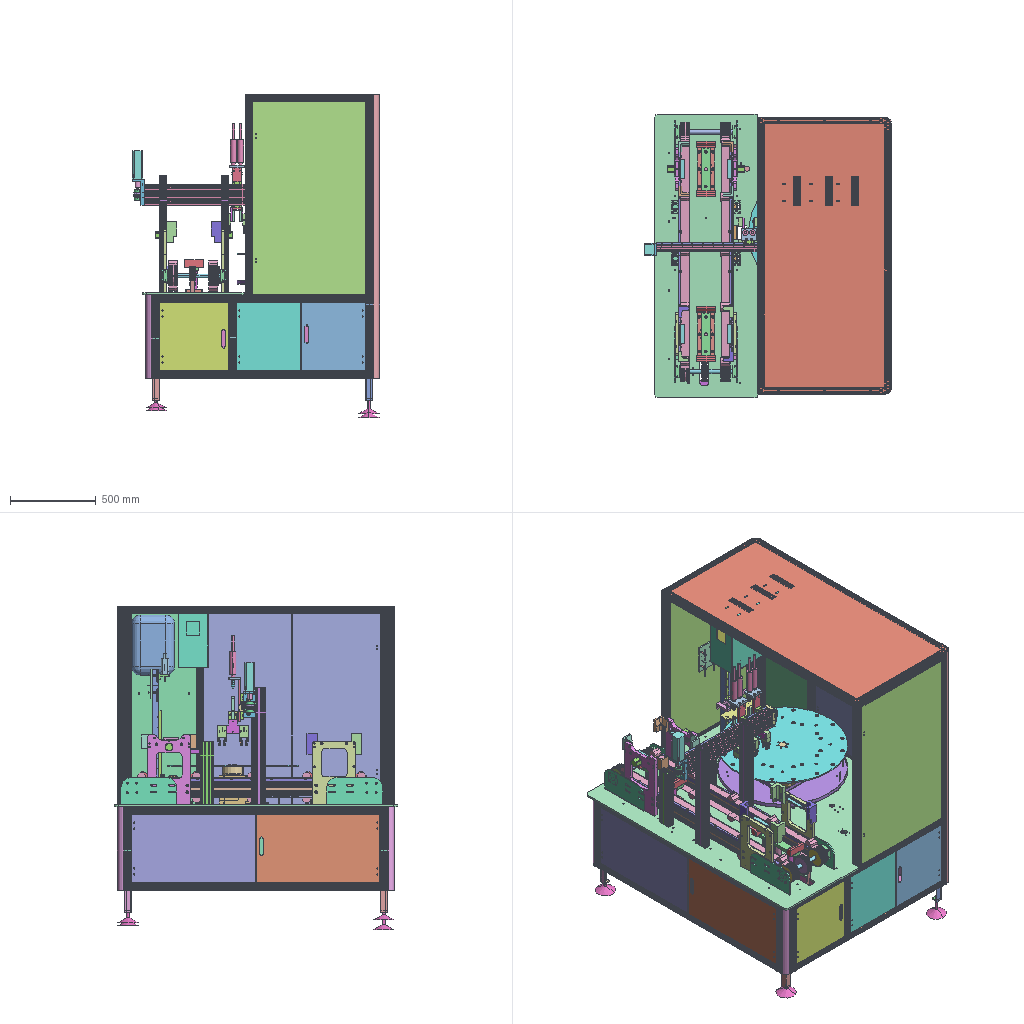Assembly | SolidWorks | 147 different items | 355 placed | box 1437 x 1650 x 1881 mm
Parts list (item | name | quantity | parent item):
1 | 1121x512x10 | x2 | in 72
2 | 1121x654x10 | x2 | in 72
3 | 12X20带轮外购加工件 | x2 | in 145, 146
4 | 12X65轴HL-TSJKD-03.3-2.1-2 | x1 | in 146
5 | 12X80轴HL-TSJKD-03.3-2.1-1 | x1 | in 145
6 | 6205轴承-外购件 | x8 | in 18, 20
7 | 6205轴承座-外购件 | x4 | in 18, 20
8 | 80DF+0.55KW普通电机+050减速机(2018-5-28)  (subassembly) | x1 | in 72
9 | 80DF+0.55KW普通电机+050减速机(2018-5-28) .stp (subassembly) | x1 | -
10 | 80针HL-TSJKD-04.4-5 | x8 | in 86
11 | CDM2B20-100Z-XC8B双杆双作用气缸-外购件 | x4 | in 79
12 | DNCJ 32X35-20-PPV-A气缸-外购件 | x1 | in 86
13 | DNCJ 32X60-20-PPV-A气缸外购件 | x1 | in 86
14 | HL-TSJKD-02.1工作台框架 (subassembly) | x1 | in 72
15 | MHZ2-20D-M9BW气缸 -外购件 | x8 | in 80, 81
16 | 三针绝缘板HL-TSJKD-04.4-1 | x1 | in 86
17 | 上料系统HL-TSJKD-03 (subassembly) | x1 | -
18 | 主动部件装配HL-TSJKD-03.1-2 (subassembly) | x1 | in 17
19 | 从动轴-353HL-TSJKD-03.1-3.1 | x1 | in 20
20 | 从动部件HL-TSJKD-03.1-3 (subassembly) | x1 | in 17
21 | 传动组件装配HL-TSJKD-03.3-2.2 (subassembly) | x2 | in 81
22 | 伺服电机-外购件ECMA-C20604RS带刹车带油封 | x1 | in 145
23 | 伺服电机联轴器-外购件 | x1 | in 145
24 | 储物柜侧门HL-TSJKD-02.5-4 | x1 | in 72
25 | 储物柜右柜门HL-TSJKD-02.5-3 | x1 | in 72
26 | 储物柜左柜门HL-TSJKD-02.5-2 | x1 | in 72
27 | 储物柜柜体HL-TSJKD-02.5-1 | x1 | in 72
28 | 光圆HL-TSJKD-03.2-2.2-3 | x4 | in 52
29 | 光敏柜柜体HL-TSJKD-02.4-1 | x1 | in 72
30 | 光敏柜盖板HL-TSJKD-02.4-2 | x1 | in 72
31 | 包电柜右门HL-TSJKD-02.8-3 | x1 | in 147
32 | 包电柜左门HL-TSJKD-02.8-2 | x1 | in 147
33 | 包电柜柜体HL-TSJKD-02.8-1 | x1 | in 147
34 | 半圆弧铝型材-1650HL-TSJKD-02.1-2.11 | x2 | in 128
35 | 半圆弧铝型材-485HL-TSJKD-02.1-2.12 | x2 | in 128
36 | 压力表盖板HL-TSJKD-02.9-2 | x1 | in 72
37 | 压皮带块1HL-TSJKD-03.3-5.1 | x2 | in 81
38 | 压皮带块2-1HL-TSJKD-03.3-5.2-1(2) | x2 | in 40
39 | 压皮带块2-2HL-TSJKD-03.3-5.2-2 | x2 | in 40
40 | 压皮带块2装配HL-TSJKD-03.3-5.2 (subassembly) | x2 | in 81
41 | 去油毛刷支架HL-TSJKD-06.2 | x10 | in 88
42 | 同步带HTD5M-3200-48-外购加工件  | x2 | in 17
43 | 同步带（HTD 750-5m）-外购件 | x1 | in 17
44 | 同步轮5m-af-30齿-27 | x1 | in 107
45 | 同步轮5m-af-70齿-27-外购加工件 | x1 | in 18
46 | 同步轮5m-af-70齿-50-外购加工件 | x2 | in 18
47 | 同步轮5m-af-70齿-50无键槽-外购加工件 | x2 | in 20
48 | 喇叭脚 | x4 | in 72
49 | 圆盘HL-TSJKD-05.1 | x1 | in 51
50 | 圆盘支撑HL-TSJKD-05.2 | x1 | in 51
51 | 圆盘机构HL-TSJKD-05 (subassembly) | x1 | -
52 | 塑料盆导向托架装配HL-TSJKD-03.2-2.2 (subassembly) | x2 | in 17
53 | 塑料盆搭扣HL-TSJKD-03.2-2.1 (subassembly) | x4 | in 17
54 | 塑料盆搭扣体HL-TSJKD-03.2-2.1-1 | x4 | in 53
55 | 塑料盆搭扣座HL-TSJKD-03.2-2.1-3 | x8 | in 53
56 | 塑料盆搭扣轴HL-TSJKD-03.2-2.1-2 | x4 | in 53
57 | 夹爪HL-TSJKD-03.3-4.1 | x14 | in 80
58 | 夹爪橡胶套-外购件 | x14 | in 80
59 | 实体1.stp | x1 | -
60 | 实体2.stp | x1 | -
61 | 实体3.stp | x1 | -
62 | 实体4.stp | x1 | -
63 | 导轨216.5HL-TSJKD-03.3-3.5 | x4 | in 85
64 | 导轨720HL-TSJKD-03.3-2.2-1 | x2 | in 21
65 | 导轨固定架HL-TSJKD-03.3-3.3 | x2 | in 85
66 | 尼龙导向角HL-TSJKD-03.2-3.1-1 | x2 | in 17
67 | 尼龙导向角切口HL-TSJKD-03.2-3.1-3 | x2 | in 17
68 | 尼龙导向角切口镜像HL-TSJKD-03.2-3.1-4 | x2 | in 17
69 | 尼龙导向角镜像HL-TSJKD-03.2-3.1-2 | x2 | in 17
70 | 尼龙托板HL-TSJKD-03.1-1.5 | x4 | in 17
71 | 工作台气缸固定板HL-TSJKD-02.3 | x2 | in 72
72 | 工作台装配体HL-TSJKD-02 (subassembly) | x1 | in 17
73 | 工作台铝板（底板）HL-TSJKD-02.2 | x1 | in 72
74 | 带轮固定板1HL-TSJKD-03.3-1.4 | x1 | in 120
75 | 带轮固定板2HL-TSJKD-03.3-1.5 | x1 | in 120
76 | 悬挂油箱盖板HL-TSJKD-02.9-1 | x1 | in 72
77 | 托架导向HL-TSJKD-03.2-2.2-2 | x4 | in 52
78 | 托架导向座HL-TSJKD-03.2-2.2-1 | x2 | in 52
79 | 执行件 (subassembly) | x4 | in 81
80 | 执行末端HL-TSJKD-03.3-4 (subassembly) | x7 | in 81
81 | 抓取机构HL-TSJKD-03.3 (subassembly) | x1 | in 17
82 | 抓取立柱铝型材80X40-680HL-TSJKD-03.3-1.1 | x2 | in 120
83 | 抓取部件1HL-TSJKD-03.3-3.2 | x2 | in 85
84 | 抓取部件HL-TSJKD-03.3-3.1 | x2 | in 85
85 | 抓取部分HL-TSJKD-03.3-3 (subassembly) | x2 | in 81
86 | 检测跳火工装HL-TSJKD-04 (subassembly) | x1 | -
87 | 毛刷托盘HL-TSJKD-06.1 | x1 | in 88
88 | 毛刷机构HL-TSJKD-06 (subassembly) | x1 | -
89 | 气缸-SDA 25X20-B-外购件 | x2 | in 17
90 | 气缸DNC50x230 PPV A-外购件 | x2 | in 17
91 | 气缸固定架HL-TSJKD-03.3-3.4 | x4 | in 85
92 | 气缸垫块HL-TSJKD-04.3-2 | x2 | in 86
93 | 油杯HL-TSJKD-04.5-2 | x4 | in 86
94 | 油杯托槽HL-TSJKD-04.5-1 | x1 | in 86
95 | 油槽托架HL-TSJKD-04.2-1 | x2 | in 86
96 | 油箱-304加厚方型10L0.8厚-外购件 | x1 | -
97 | 油箱-304加厚方型20L0.8厚-外购件 | x1 | -
98 | 油箱右柜门HL-TSJKD-02.7-1 | x1 | in 72
99 | 油箱左柜门HL-TSJKD-02.7-2 | x1 | in 72
100 | 浮动接头-外购件 FJ1008 M8x1.25 | x4 | in 79
101 | 滑块-外购件（TRH15A直线导轨块） | x12 | in 21, 85, 86
102 | 滑块支座HL-TSJKD-04.3-1 | x2 | in 86
103 | 电机ECM-B3M-C20604RS1-外购件 | x1 | in 107
104 | 电机支架1HL-TSJKD-03.1-4.1-1 | x2 | in 106
105 | 电机支架2HL-TSJKD-03.1-4.1-2 | x1 | in 106
106 | 电机支架HL-TSJKD-03.1-4.1 (subassembly) | x1 | in 107
107 | 电机组件HL-TSJKD-03.1-4 (subassembly) | x1 | in 17
108 | 电极头HL-TSJKD-04.4-6 | x4 | in 86
109 | 电极头触点导电块HL-TSJKD-04.4-7 | x4 | in 86
110 | 电极座HL-TSJKD-04.4-4 | x8 | in 86
111 | 电气柜右柜体HL-TSJKD-02.6-1.2 | x1 | in 72
112 | 电气柜右柜门HL-TSJKD-02.6-3.DWG | x2 | in 72
113 | 电气柜左柜体HL-TSJKD-02.6-1.1 | x1 | in 72
114 | 电气柜左柜门HL-TSJKD-02.6-2 | x2 | in 72
115 | 直线轴承装配 (subassembly) | x4 | in 17
116 | 直线轴承轴 | x4 | in 115
117 | 直线轴承轴座-25&35x130有肩轴套（浙江茅）- | x4 | in 115
118 | 立式KP001轴承套-外购件 | x4 | in 120
119 | 立柱铝型材HL-TSJKD-04.1 | x1 | in 86
120 | 结构框架装配HL-TSJKD-03.3-1 (subassembly) | x1 | in 81
121 | 绝缘卡件HL-TSJKD-04.4-3.2 | x2 | in 123
122 | 绝缘板HL-TSJKD-04.4-3.1 | x1 | in 123
123 | 绝缘板部件HL-TSJKD-04.4-3 (subassembly) | x1 | in 86
124 | 角铁框架HL-TSJKD-02.1-1 | x1 | in 14
125 | 跳火导轨495-外购加工件（配合TRH15A） | x2 | in 86
126 | 轴-353HL-TSJKD-03.1-2.1 | x1 | in 18
127 | 轴承安装板HL-TSJKD-03.1-1.6 | x4 | in 17
128 | 铝合金框架装配HL-TSJKD-02.1-2 (subassembly) | x1 | in 14
129 | 铝型材40X40-1125HL-TSJKD-02.1-2.1 | x1 | in 128
130 | 铝型材40X40-1164HL-TSJKD-02.1-2.2 | x2 | in 128
131 | 铝型材40X40-1200HL-TSJKD-02.1-2.3 | x4 | in 128
132 | 铝型材40X40-1450HL-TSJKD-02.1-2.4 | x5 | in 128
133 | 铝型材40X40-1530HL-TSJKD-02.1-2.5 | x1 | in 128
134 | 铝型材40X40-1650HL-TSJKD-02.1-2.6 | x4 | in 128
135 | 铝型材40X40-170HL-TSJKD-02.1-2.7 | x3 | in 128
136 | 铝型材40X40-405HL-TSJKD-02.1-2.8 | x2 | in 128
137 | 铝型材40X40-485HL-TSJKD-02.1-2.9 | x4 | in 128
138 | 铝型材40X40-658HL-TSJKD-02.1-2.10 | x2 | in 128
139 | 铝型材40x120-720HL-TSJKD-03.3-1.2 | x1 | in 120
140 | 铝型材80X40-1260HL-TSJKD-03.1-1.4 | x2 | in 17
141 | 铝型材80X40-366HL-TSJKD-03.1-1.3 | x2 | in 17
142 | 铝板366x250x20HL-TSJKD-03.1-1.2 | x2 | in 17
143 | 铝板406X250X20HL-TSJKD-03.1-1.1 | x2 | in 17
144 | 顶部盖板HL-TSJKD-02.9-3 | x1 | in 72
145 | 驱动源主动部件装配HL-TSJKD-03.3-2.1 (subassembly) | x1 | in 81
146 | 驱动源从动部件装配HL-TSJKD-03.3-2.1 (subassembly) | x1 | in 81
147 | 高压包电柜装配HL-TSJKD-02.8 (subassembly) | x1 | in 72
Mates (type | each side: item.copy, entity, surface, feature), first 515 of 572 lines:
In the top assembly
Coincident | 73.1 face plane 凸台-拉伸1 | 119.1 face plane 凸台-拉伸1 | 2 times
DistanceDim | 119.1 face plane 凸台-拉伸2 | 73.1 face plane 凸台-拉伸1
DistanceDim | 73.1 face plane 凸台-拉伸1 | 87.1 face plane 凸台-拉伸1
Concentric | 49.1 face cylinder 凸台-拉伸1 | 87.1 face cylinder 边线-法兰1
Coincident | 124.1 edge | 97.1 face plane 凸台-拉伸1
Coincident | 124.1 face plane 等边角钢gb／t 9787-1988 40X40X5 型号：4#(1) | 97.1 face plane 凸台-拉伸1 | 2 times
Coincident | 76.1 face plane 基体-法兰1 | 96.1 face plane 凸台-拉伸1
Coincident | 76.1 face plane 边线-法兰1 | 96.1 face plane 凸台-拉伸1
In subassembly 88
Coincident | 87.2 face plane 切除-拉伸1 | 41.1 face plane 凸台-拉伸1 | 3 times
Coincident | 87.2 face plane 切除-拉伸1 | 41.2 face plane 凸台-拉伸1 | 3 times
In subassembly 17
Coincident | 73.2 face plane 凸台-拉伸1 | 142.1 face plane 凸台-拉伸1
Concentric | 73.2 face cylinder 凸台-拉伸1 | 142.1 face cylinder M8 螺纹孔2 | 2 times
Coincident | 73.2 face plane 凸台-拉伸1 | 142.2 face plane 凸台-拉伸1
Concentric | 73.2 face cylinder 凸台-拉伸1 | 142.2 face cylinder M8 螺纹孔2 | 2 times
Coincident | 73.2 face plane 凸台-拉伸1 | 143.1 face plane 切除-拉伸5
Coincident | 73.2 face plane 凸台-拉伸1 | 143.2 face plane 切除-拉伸5
Concentric | 73.2 face cylinder 凸台-拉伸1 | 143.2 face cylinder M8 螺纹孔4 | 2 times
Concentric | 73.2 face cylinder 凸台-拉伸1 | 143.1 face cylinder M8 螺纹孔4 | 2 times
Coincident | 73.2 face plane 凸台-拉伸1 | 127.1 face plane 凸台-拉伸2
Coincident | 142.1 face plane 凸台-拉伸1 | 127.1 face plane 凸台-拉伸1
Slot | 127.1 face plane 切除-拉伸1 | 142.1 face cylinder M8 螺纹孔1
Coincident | 73.2 face plane 凸台-拉伸1 | 127.2 face plane 凸台-拉伸2
Coincident | 142.2 face plane 凸台-拉伸1 | 127.2 face plane 凸台-拉伸1
Slot | 142.2 face cylinder M8 螺纹孔1 | 127.2 face plane 切除-拉伸1
Coincident | 127.1 face plane 凸台-拉伸2 | 127.2 face plane 凸台-拉伸2
Coincident | 73.2 face plane 凸台-拉伸1 | 127.3 face plane 凸台-拉伸2
Coincident | 73.2 face plane 凸台-拉伸1 | 127.4 face plane 凸台-拉伸2
Coincident | 143.1 face plane 凸台-拉伸1 | 127.4 face plane 凸台-拉伸1
Coincident | 143.2 face plane 凸台-拉伸1 | 127.3 face plane 凸台-拉伸1
Slot | 127.3 face plane 切除-拉伸1 | 143.2 face cylinder M8 螺纹孔3
Coincident | 127.4 face plane 凸台-拉伸2 | 127.3 face plane 凸台-拉伸2
Slot | 127.4 face plane 切除-拉伸1 | 143.1 face cylinder M8 螺纹孔3
Coincident | 142.2 face plane 凸台-拉伸1 | 140.1 face plane 凸台-拉伸1
Coincident | 143.1 face plane 凸台-拉伸1 | 140.2 face plane 凸台-拉伸1
Coincident | 143.2 face plane 凸台-拉伸1 | 140.1 face plane 凸台-拉伸1
DistanceDim | 140.1 face plane 凸台-拉伸1 | 143.2 face plane 凸台-拉伸1
Coincident | 140.2 face plane 凸台-拉伸1 | 140.1 face plane 凸台-拉伸1 | 2 times
Tangent | 143.2 face cylinder 打孔尺寸(%根据)内六角圆柱头螺钉的类型1 | 140.1 face plane 凸台-拉伸1
Coincident | 140.2 face plane 凸台-拉伸1 | 70.1 face plane 凸台-拉伸1
Coincident | 140.1 edge | 70.1 edge
Tangent | 140.1 face plane 凸台-拉伸1 | 70.1 face cylinder 打孔尺寸(%根据)内六角圆柱头螺钉的类型1
Coincident | 70.2 edge | 70.1 edge
Coincident | 70.2 face plane 凸台-拉伸1 | 70.1 face plane 凸台-拉伸1
Parallel | 140.2 face plane 凸台-拉伸1 | 70.3 face plane 凸台-拉伸1
Coincident | 140.2 face plane 凸台-拉伸1 | 70.3 face plane 凸台-拉伸1
Tangent | 140.2 face plane 凸台-拉伸1 | 70.3 face cylinder 打孔尺寸(%根据)内六角圆柱头螺钉的类型1
Coincident | 140.2 edge | 70.3 edge
Coincident | 70.4 edge | 70.3 edge
Coincident | 70.3 face plane 凸台-拉伸1 | 70.4 face plane 凸台-拉伸1
Coincident | 141.1 face plane 凸台-拉伸1 | 141.2 face plane 凸台-拉伸1 | 2 times
Coincident | 140.1 face plane 凸台-拉伸1 | 141.2 face plane 凸台-拉伸1
Coincident | 140.2 face plane 凸台-拉伸1 | 141.1 face plane 凸台-拉伸1
Coincident | 73.2 face plane 凸台-拉伸1 | 141.1 face plane 凸台-拉伸1
DistanceDim | 141.1 face plane 凸台-拉伸1 | 143.1 face plane 凸台-拉伸1
Coincident | 70.4 face plane 凸台-拉伸1 | 42.1 face plane 凸台-拉伸1
Coincident | 127.1 face plane 凸台-拉伸1 | 7.1 face plane 凸台-拉伸1
Concentric | 127.1 face cylinder 切除-拉伸1 | 7.1 face cylinder M8 六角头螺栓的柱形沉头孔1 | 2 times
Concentric | 127.2 face cylinder 切除-拉伸1 | 7.2 face cylinder M8 六角头螺栓的柱形沉头孔1 | 2 times
Concentric | 42.2 face cylinder 凸台-拉伸1 | 46.1 face cylinder 凸台-拉伸2
Coincident | 127.3 face plane 凸台-拉伸1 | 7.3 face plane 凸台-拉伸1
Concentric | 127.3 face cylinder 切除-拉伸1 | 7.3 face cylinder M8 六角头螺栓的柱形沉头孔1 | 3 times
Concentric | 127.4 face cylinder 切除-拉伸1 | 7.4 face cylinder M8 六角头螺栓的柱形沉头孔1 | 2 times
Concentric | 42.1 face cylinder 凸台-拉伸1 | 47.1 face cylinder 凸台-拉伸3
DistanceDim | 42.1 face plane 凸台-拉伸1 | 46.2 face plane 凸台-拉伸3
Coincident | 73.2 face plane 凸台-拉伸1 | 105.1 face plane 基体-法兰1
Slot | 105.1 face plane 切除-拉伸1 | 73.2 face cylinder M8 螺纹孔1
Slot | 73.2 face cylinder M8 螺纹孔1 | 105.1 face plane 切除-拉伸1
Coincident | 45.1 face plane 凸台-拉伸3 | 44.1 face plane 凸台-拉伸2
Concentric | 143.2 face cylinder 切除-拉伸4 | 89.1 face cylinder 凸台-拉伸3
Coincident | 143.2 face plane 凸台-拉伸1 | 89.1 face plane 凸台-拉伸2
Concentric | 143.1 face cylinder 切除-拉伸4 | 89.2 face cylinder 凸台-拉伸3
Coincident | 143.1 face plane 凸台-拉伸1 | 89.2 face plane 凸台-拉伸2
Concentric | 71.1 face cylinder 凸台-拉伸1 | 90.1 face cylinder 凸台-拉伸4
Coincident | 71.1 face plane 凸台-拉伸1 | 90.1 face plane 凸台-拉伸1
Concentric | 71.2 face cylinder 凸台-拉伸1 | 90.2 face cylinder 凸台-拉伸4
Coincident | 71.2 face plane 凸台-拉伸1 | 90.2 face plane 凸台-拉伸1
Coincident | 142.2 face plane 凸台-拉伸1 | 55.1 face plane 凸台-拉伸1
Coincident | 142.1 face plane 凸台-拉伸1 | 55.2 face plane 凸台-拉伸1
Concentric | 142.2 face cylinder 切除-拉伸5 | 55.1 face cylinder M8 螺纹孔1
Concentric | 142.2 face cylinder 切除-拉伸5 | 55.3 face cylinder M8 螺纹孔1
Concentric | 142.1 face cylinder 切除-拉伸5 | 55.2 face cylinder M8 螺纹孔1
Concentric | 142.1 face cylinder 切除-拉伸5 | 55.4 face cylinder M8 螺纹孔1
Coincident | 143.1 face plane 凸台-拉伸1 | 54.1 face plane 切除-拉伸1
Concentric | 143.1 face cylinder 打孔尺寸(%根据)内六角圆柱头螺钉的类型3 | 55.5 face cylinder M8 螺纹孔1
Concentric | 143.1 face cylinder 打孔尺寸(%根据)内六角圆柱头螺钉的类型3 | 55.6 face cylinder M8 螺纹孔1
Coincident | 143.2 face plane 凸台-拉伸1 | 55.7 face plane 凸台-拉伸1
Concentric | 143.2 face cylinder 打孔尺寸(%根据)内六角圆柱头螺钉的类型3 | 55.7 face cylinder M8 螺纹孔1
Concentric | 143.2 face cylinder 打孔尺寸(%根据)内六角圆柱头螺钉的类型3 | 55.8 face cylinder M8 螺纹孔1
Concentric | 71.2 face cylinder 凸台-拉伸1 | 28.1 face cylinder 凸台-拉伸1
Concentric | 71.2 face cylinder 凸台-拉伸1 | 28.2 face cylinder 凸台-拉伸1
Coincident | 90.2 face plane 凸台-拉伸4 | 78.1 face plane 凸台-拉伸1
Concentric | 71.1 face cylinder 凸台-拉伸1 | 28.3 face cylinder 凸台-拉伸1
Concentric | 71.1 face cylinder 凸台-拉伸1 | 28.4 face cylinder 凸台-拉伸1
Coincident | 90.1 face plane 凸台-拉伸4 | 78.2 face plane 凸台-拉伸1
Coincident | 71.1 face plane 凸台-拉伸1 | 117.1 face plane 凸台-拉伸1
Concentric | 71.1 face cylinder M5 螺纹孔1 | 117.1 face cylinder M5 螺纹孔1 | 2 times
Coincident | 71.2 face plane 凸台-拉伸1 | 117.2 face plane 凸台-拉伸1
Coincident | 71.2 face plane 凸台-拉伸1 | 117.3 face plane 凸台-拉伸1
Coincident | 71.1 face plane 凸台-拉伸1 | 117.4 face plane 凸台-拉伸1
Concentric | 28.4 face cylinder 凸台-拉伸1 | 116.1 face cylinder 凸台-拉伸2
Concentric | 28.1 face cylinder 凸台-拉伸1 | 116.2 face cylinder 凸台-拉伸2
Concentric | 28.2 face cylinder 凸台-拉伸1 | 116.3 face cylinder 凸台-拉伸2
Concentric | 143.1 face cylinder M8 螺纹孔1 | 66.1 face cylinder 打孔尺寸(%根据)内六角圆柱头螺钉的类型2 | 2 times
Coincident | 143.1 face plane 凸台-拉伸1 | 66.1 face plane 切除-拉伸2
Concentric | 143.2 face cylinder M8 螺纹孔1 | 66.2 face cylinder 打孔尺寸(%根据)内六角圆柱头螺钉的类型2 | 2 times
Coincident | 143.2 face plane 凸台-拉伸1 | 66.2 face plane 切除-拉伸2
Concentric | 143.2 face cylinder M8 螺纹孔1 | 69.1 face cylinder 打孔尺寸(%根据)内六角圆柱头螺钉的类型2 | 2 times
Coincident | 143.2 face plane 凸台-拉伸1 | 69.1 face plane 切除-拉伸2
Concentric | 142.1 face cylinder M8 螺纹孔1 | 67.1 face cylinder 打孔尺寸(%根据)内六角圆柱头螺钉的类型3 | 2 times
Coincident | 142.1 face plane 凸台-拉伸1 | 67.1 face plane 切除-拉伸5
Concentric | 142.1 face cylinder M8 螺纹孔1 | 68.1 face cylinder 打孔尺寸(%根据)内六角圆柱头螺钉的类型3 | 2 times
Coincident | 142.1 face plane 凸台-拉伸1 | 68.1 face plane 切除-拉伸5
Concentric | 142.2 face cylinder M8 螺纹孔1 | 67.2 face cylinder 打孔尺寸(%根据)内六角圆柱头螺钉的类型3 | 2 times
Coincident | 142.2 face plane 凸台-拉伸1 | 67.2 face plane 切除-拉伸5
Concentric | 142.2 face cylinder M8 螺纹孔1 | 68.2 face cylinder 打孔尺寸(%根据)内六角圆柱头螺钉的类型3 | 2 times
Coincident | 142.2 face plane 凸台-拉伸1 | 68.2 face plane 切除-拉伸5
Coincident | 143.1 face plane 凸台-拉伸1 | 69.2 face plane 切除-拉伸2
Concentric | 143.1 face cylinder M8 螺纹孔1 | 69.2 face cylinder 打孔尺寸(%根据)内六角圆柱头螺钉的类型2 | 2 times
Coincident | 73.2 face plane 凸台-拉伸1 | 82.1 face plane 凸台-拉伸1
Coincident | 140.2 face plane 凸台-拉伸1 | 82.1 face plane 凸台-拉伸1
DistanceDim | 82.1 face plane 凸台-拉伸1 | 73.2 face plane 凸台-拉伸1
Concentric | 45.1 face cylinder 凸台-拉伸2 | 43.1 face cylinder 扫描1
DistanceDim | 43.1 face plane 扫描1 | 45.1 face plane 凸台-拉伸2
In subassembly 72
Coincident | 124.2 face plane 等边角钢gb／t 9787-1988 40X40X5 型号：4#(1) | 73.3 face plane 凸台-拉伸1 | 2 times
DistanceDim | 124.2 face plane 等边角钢gb／t 9787-1988 40X40X5 型号：4#(1) | 73.3 face plane 凸台-拉伸1
Coincident | 73.3 face plane 凸台-拉伸1 | 71.3 face plane 凸台-拉伸1
Coincident | 73.3 face plane 凸台-拉伸1 | 71.4 face plane 凸台-拉伸1
Concentric | 73.3 face cylinder M8 螺纹孔1 | 71.4 face cylinder 切除-拉伸1
Parallel | 73.3 face cylinder M8 螺纹孔1 | 71.4 face cylinder 凸台-拉伸1
Concentric | 73.3 face cylinder M8 螺纹孔1 | 71.3 face cylinder 凸台-拉伸1
Concentric | 73.3 face cylinder M8 螺纹孔1 | 71.3 face cylinder 切除-拉伸1
Coincident | 124.2 face plane 等边角钢gb／t 9787-1988 40X40X5 型号：4#(1) | 29.1 face plane 边线-法兰1
Coincident | 124.2 edge | 29.1 face plane 边线-法兰2
Coincident | 124.2 edge | 29.1 face plane 边线-法兰1
DistanceDim | 30.1 face plane 斜接法兰1 | 131.1 face plane 铝型材 40 X 40B X R4.5(1)
DistanceDim | 30.1 face plane 斜接法兰1 | 136.1 face plane 铝型材 40 X 40B X R4.5(1)
Coincident | 136.1 face plane 铝型材 40 X 40B X R4.5(1) | 30.1 face plane 基体-法兰1
Coincident | 124.2 face plane 等边角钢gb／t 9787-1988 40X40X5 型号：4#(1) | 27.1 face plane 基体-法兰1
Coincident | 124.2 edge | 27.1 face plane 边线-法兰1 | 2 times
Coincident | 26.1 face plane 基体-法兰1 | 25.1 face plane 基体-法兰1
Coincident | 26.1 face plane 斜接法兰1 | 25.1 face plane 斜接法兰1
DistanceDim | 26.1 face plane 斜接法兰1 | 131.2 face plane 铝型材 40 X 40B X R4.5(1)
DistanceDim | 26.1 face plane 斜接法兰1 | 136.2 face plane 铝型材 40 X 40B X R4.5(1)
DistanceDim | 25.1 face plane 斜接法兰1 | 134.1 face plane 铝型材 40 X 40B X R4.5(1)
Coincident | 26.1 face plane 基体-法兰1 | 24.1 face plane 基体-法兰1
Coincident | 26.1 face plane 斜接法兰1 | 24.1 face plane 斜接法兰1
DistanceDim | 24.1 face plane 斜接法兰1 | 137.1 face plane 铝型材 40 X 40B X R4.5(1)
Coincident | 124.2 face plane 等边角钢gb／t 9787-1988 40X40X5 型号：4#(1) | 113.1 face plane 基体-法兰1
Coincident | 124.2 edge | 113.1 face plane 边线-法兰1
Coincident | 124.2 edge | 113.1 face plane 基体-法兰1
Coincident | 124.2 edge | 111.1 face plane 基体-法兰1
Coincident | 124.2 face plane 等边角钢gb／t 9787-1988 40X40X5 型号：4#(1) | 111.1 face plane 基体-法兰1
DistanceDim | 29.1 face plane 基体-法兰1 | 111.1 face plane 基体-法兰1
DistanceDim | 112.1 face plane 斜接法兰1 | 137.2 face plane 铝型材 40 X 40B X R4.5(1)
DistanceDim | 112.1 face plane 斜接法兰1 | 132.1 face plane 铝型材 40 X 40B X R4.5(1)
Coincident | 137.2 face plane 铝型材 40 X 40B X R4.5(1) | 112.1 face plane 基体-法兰1
Coincident | 132.2 face plane 铝型材 40 X 40B X R4.5(1) | 112.2 face plane 基体-法兰1
DistanceDim | 112.2 face plane 斜接法兰1 | 134.2 face plane 铝型材 40 X 40B X R4.5(1)
DistanceDim | 112.2 face plane 斜接法兰1 | 132.3 face plane 铝型材 40 X 40B X R4.5(1)
Coincident | 137.3 face plane 铝型材 40 X 40B X R4.5(1) | 114.1 face plane 基体-法兰1
DistanceDim | 114.1 face plane 斜接法兰1 | 137.3 face plane 铝型材 40 X 40B X R4.5(1)
DistanceDim | 114.1 face plane 斜接法兰1 | 132.1 face plane 铝型材 40 X 40B X R4.5(1)
Coincident | 134.3 face plane 铝型材 40 X 40B X R4.5(1) | 114.2 face plane 基体-法兰1
DistanceDim | 114.2 face plane 斜接法兰1 | 134.3 face plane 铝型材 40 X 40B X R4.5(1)
DistanceDim | 114.2 face plane 斜接法兰1 | 132.3 face plane 铝型材 40 X 40B X R4.5(1)
Coincident | 134.4 face plane 铝型材 40 X 40B X R4.5(1) | 99.1 face plane 基体-法兰1
DistanceDim | 99.1 face plane 斜接法兰1 | 134.4 face plane 铝型材 40 X 40B X R4.5(1)
DistanceDim | 99.1 face plane 斜接法兰1 | 131.1 face plane 铝型材 40 X 40B X R4.5(1)
Coincident | 131.3 face plane 铝型材 40 X 40B X R4.5(1) | 98.1 face plane 基体-法兰1
DistanceDim | 98.1 face plane 斜接法兰1 | 131.1 face plane 铝型材 40 X 40B X R4.5(1)
DistanceDim | 98.1 face plane 斜接法兰1 | 136.1 face plane 铝型材 40 X 40B X R4.5(1)
Coincident | 135.1 face plane 铝型材 40 X 40B X R4.5(1) | 33.1 face plane 斜接法兰1
DistanceDim | 33.1 face plane 斜接法兰1 | 135.1 face plane 铝型材 40 X 40B X R4.5(1)
DistanceDim | 124.2 edge | 36.1 face plane 凸台-拉伸1
Coincident | 124.2 face plane 等边角钢gb／t 9787-1988 40X40X5 型号：4#(1) | 36.1 face plane 凸台-拉伸1
Coincident | 113.1 face plane 边线-法兰1 | 36.1 face plane 凸台-拉伸1
Coincident | 129.1 face plane 铝型材 40 X 40B X R4.5(1) | 76.2 face plane 基体-法兰1
DistanceDim | 76.2 face plane 边线-法兰1 | 132.4 face plane 铝型材 40 X 40B X R4.5(1)
DistanceDim | 76.2 face plane 边线-法兰1 | 134.2 face plane 铝型材 40 X 40B X R4.5(1)
Coincident | 138.1 face plane 铝型材 40 X 40B X R4.5(1) | 144.1 face plane 凸台-拉伸1
DistanceDim | 144.1 face plane 凸台-拉伸1 | 138.1 face plane 铝型材 40 X 40B X R4.5(1)
DistanceDim | 144.1 face plane 凸台-拉伸1 | 134.3 face plane 铝型材 40 X 40B X R4.5(1)
Coincident | 134.3 face plane 铝型材 40 X 40B X R4.5(1) | 1.1 face plane 凸台-拉伸1 | 2 times
DistanceDim | 1.1 face plane 凸台-拉伸1 | 132.4 face plane 铝型材 40 X 40B X R4.5(1)
DistanceDim | 1.1 face plane 凸台-拉伸1 | 134.3 face plane 铝型材 40 X 40B X R4.5(1)
Coincident | 129.1 face plane 铝型材 40 X 40B X R4.5(1) | 1.2 face plane 凸台-拉伸1
DistanceDim | 1.2 face plane 凸台-拉伸1 | 132.4 face plane 铝型材 40 X 40B X R4.5(1)
DistanceDim | 1.2 face plane 凸台-拉伸1 | 129.1 face plane 铝型材 40 X 40B X R4.5(1)
Coincident | 134.4 face plane 铝型材 40 X 40B X R4.5(1) | 2.1 face plane 凸台-拉伸1
DistanceDim | 2.1 face plane 凸台-拉伸1 | 138.2 face plane 铝型材 40 X 40B X R4.5(1)
DistanceDim | 2.1 face plane 凸台-拉伸1 | 130.1 face plane 铝型材 40 X 40B X R4.5(1)
Coincident | 130.2 face plane 铝型材 40 X 40B X R4.5(1) | 2.2 face plane 凸台-拉伸1
DistanceDim | 2.2 face plane 凸台-拉伸1 | 130.2 face plane 铝型材 40 X 40B X R4.5(1)
DistanceDim | 2.2 face plane 凸台-拉伸1 | 138.1 face plane 铝型材 40 X 40B X R4.5(1)
Concentric | 124.2 face cylinder M16 螺纹孔1 | 48.1 face cylinder 旋转1
DistanceDim | 48.1 face plane 旋转1 | 124.2 face plane 凸台-拉伸1
Concentric | 124.2 face cylinder M16 螺纹孔1 | 48.2 face cylinder 旋转1
Concentric | 124.2 face cylinder M16 螺纹孔1 | 48.3 face cylinder 旋转1
Concentric | 124.2 face cylinder M16 螺纹孔1 | 48.4 face cylinder 旋转1
In subassembly 147
Coincident | 33.2 face plane 斜接法兰1 | 31.1 face plane 基体-法兰1
Coincident | 33.2 face plane 斜接法兰1 | 32.1 face plane 基体-法兰1
DistanceDim | 31.1 face plane 斜接法兰1 | 33.2 face plane 斜接法兰1 | 2 times
DistanceDim | 32.1 face plane 斜接法兰1 | 33.2 face plane 斜接法兰1 | 2 times
In subassembly 14
Coincident | 124.3 face plane 等边角钢gb／t 9787-1988 40X40X5 型号：4#(1) | 131.4 face plane 铝型材 40 X 40B X R4.5(1) | 2 times
Coincident | 124.3 face plane 等边角钢gb／t 9787-1988 40X40X5 型号：4#(1) | 132.5 face plane 铝型材 40 X 40B X R4.5(1)
In subassembly 128
Coincident | 34.1 face plane 凸台-拉伸1 | 34.2 face plane 凸台-拉伸1
Coincident | 34.1 face plane 凸台-拉伸1 | 134.5 face plane 铝型材 40 X 40B X R4.5(1) | 3 times
Coincident | 34.1 face plane 凸台-拉伸1 | 134.6 face plane 铝型材 40 X 40B X R4.5(1) | 2 times
Coincident | 134.5 edge | 134.6 face plane 铝型材 40 X 40B X R4.5(1)
Coincident | 34.2 face plane 凸台-拉伸1 | 134.7 face plane 铝型材 40 X 40B X R4.5(1) | 3 times
Coincident | 34.2 face plane 凸台-拉伸1 | 134.8 face plane 铝型材 40 X 40B X R4.5(1)
Coincident | 134.7 edge | 134.8 face plane 铝型材 40 X 40B X R4.5(1)
Coincident | 134.7 face plane 铝型材 40 X 40B X R4.5(1) | 134.8 face plane 铝型材 40 X 40B X R4.5(1)
Coincident | 134.6 face plane 铝型材 40 X 40B X R4.5(1) | 132.6 face plane 铝型材 40 X 40B X R4.5(1) | 3 times
Coincident | 134.7 face plane 铝型材 40 X 40B X R4.5(1) | 132.6 face plane 铝型材 40 X 40B X R4.5(1) | 3 times
Coincident | 35.1 face plane 凸台-拉伸1 | 137.4 face plane 铝型材 40 X 40B X R4.5(1) | 3 times
Coincident | 35.1 edge | 137.5 face plane 铝型材 40 X 40B X R4.5(1)
Coincident | 35.1 face plane 凸台-拉伸1 | 137.5 face plane 铝型材 40 X 40B X R4.5(1)
Coincident | 35.1 edge | 137.5 edge
Coincident | 134.5 face plane 铝型材 40 X 40B X R4.5(1) | 137.4 face plane 铝型材 40 X 40B X R4.5(1) | 2 times
Coincident | 34.1 face plane 凸台-拉伸1 | 35.1 face plane 凸台-拉伸1
Coincident | 134.8 face plane 铝型材 40 X 40B X R4.5(1) | 137.6 face plane 铝型材 40 X 40B X R4.5(1)
Concentric | 134.7 face cylinder 切除-拉伸1 | 132.7 face cylinder 铝型材 40 X 40B X R4.5(1)
Coincident | 134.7 face plane 铝型材 40 X 40B X R4.5(1) | 132.7 face plane 铝型材 40 X 40B X R4.5(1)
Concentric | 137.4 face cylinder 切除-拉伸1 | 131.5 face cylinder 铝型材 40 X 40B X R4.5(1)
Coincident | 137.4 face plane 铝型材 40 X 40B X R4.5(1) | 131.5 face plane 铝型材 40 X 40B X R4.5(1)
Coincident | 134.5 face plane 铝型材 40 X 40B X R4.5(1) | 131.5 face plane 铝型材 40 X 40B X R4.5(1)
Coincident | 134.8 face plane 铝型材 40 X 40B X R4.5(1) | 131.6 face plane 铝型材 40 X 40B X R4.5(1)
Concentric | 134.8 face cylinder 切除-拉伸1 | 131.6 face cylinder 铝型材 40 X 40B X R4.5(1)
Coincident | 137.6 face plane 铝型材 40 X 40B X R4.5(1) | 131.6 face plane 铝型材 40 X 40B X R4.5(1) | 2 times
Coincident | 134.8 face plane 铝型材 40 X 40B X R4.5(1) | 131.7 face plane 铝型材 40 X 40B X R4.5(1)
Concentric | 134.8 face cylinder 切除-拉伸1 | 131.7 face cylinder 铝型材 40 X 40B X R4.5(1)
Coincident | 137.4 face plane 铝型材 40 X 40B X R4.5(1) | 131.8 face plane 铝型材 40 X 40B X R4.5(1)
Concentric | 137.4 face cylinder 切除-拉伸1 | 131.8 face cylinder 铝型材 40 X 40B X R4.5(1)
Coincident | 134.6 face plane 铝型材 40 X 40B X R4.5(1) | 132.8 face plane 铝型材 40 X 40B X R4.5(1)
Concentric | 134.6 face cylinder 切除-拉伸1 | 132.8 face cylinder 铝型材 40 X 40B X R4.5(1)
Coincident | 137.5 face plane 铝型材 40 X 40B X R4.5(1) | 132.9 face plane 铝型材 40 X 40B X R4.5(1)
Concentric | 137.5 face cylinder 切除-拉伸1 | 132.9 face cylinder 铝型材 40 X 40B X R4.5(1)
Coincident | 137.5 face plane 铝型材 40 X 40B X R4.5(1) | 132.10 face plane 铝型材 40 X 40B X R4.5(1)
Concentric | 137.5 face cylinder 切除-拉伸1 | 132.10 face cylinder 铝型材 40 X 40B X R4.5(1)
Coincident | 134.8 face plane 铝型材 40 X 40B X R4.5(1) | 138.3 face plane 铝型材 40 X 40B X R4.5(1)
Concentric | 134.8 face cylinder 切除-拉伸1 | 138.3 face cylinder 铝型材 40 X 40B X R4.5(1)
Coincident | 134.5 face plane 铝型材 40 X 40B X R4.5(1) | 138.4 face plane 铝型材 40 X 40B X R4.5(1)
Concentric | 134.5 face cylinder 切除-拉伸1 | 138.4 face cylinder 铝型材 40 X 40B X R4.5(1)
Concentric | 138.3 face cylinder 铝型材 40 X 40B X R4.5(1) | 130.3 face cylinder 切除-拉伸1
Coincident | 138.3 face plane 铝型材 40 X 40B X R4.5(1) | 130.3 face plane 铝型材 40 X 40B X R4.5(1)
Coincident | 138.4 face plane 铝型材 40 X 40B X R4.5(1) | 130.4 face plane 铝型材 40 X 40B X R4.5(1)
Concentric | 138.4 face cylinder 铝型材 40 X 40B X R4.5(1) | 130.4 face cylinder 切除-拉伸1
Concentric | 133.1 face cylinder 铝型材 40 X 40B X R4.5(1) | 130.4 face cylinder 切除-拉伸2
Coincident | 133.1 face plane 铝型材 40 X 40B X R4.5(1) | 130.4 face plane 铝型材 40 X 40B X R4.5(1)
Coincident | 131.5 face plane 铝型材 40 X 40B X R4.5(1) | 136.3 face plane 铝型材 40 X 40B X R4.5(1)
Concentric | 131.8 face cylinder 切除-拉伸1 | 136.3 face cylinder 铝型材 40 X 40B X R4.5(1)
Coincident | 131.6 face plane 铝型材 40 X 40B X R4.5(1) | 136.4 face plane 铝型材 40 X 40B X R4.5(1)
Concentric | 131.7 edge | 136.4 face cylinder 铝型材 40 X 40B X R4.5(1)
Coincident | 132.6 face plane 铝型材 40 X 40B X R4.5(1) | 129.2 face plane 铝型材 40 X 40B X R4.5(1)
Concentric | 132.6 face cylinder 切除-拉伸1 | 129.2 face cylinder 铝型材 40 X 40B X R4.5(1)
Coincident | 135.2 face plane 铝型材 40 X 40B X R4.5(1) | 135.3 face plane 铝型材 40 X 40B X R4.5(1) | 2 times
Coincident | 135.2 face plane 铝型材 40 X 40B X R4.5(1) | 135.4 face plane 铝型材 40 X 40B X R4.5(1) | 2 times
Coincident | 132.6 face plane 铝型材 40 X 40B X R4.5(1) | 135.4 face plane 铝型材 40 X 40B X R4.5(1)
Coincident | 137.7 face plane 铝型材 40 X 40B X R4.5(1) | 132.9 face plane 铝型材 40 X 40B X R4.5(1) | 3 times
Coincident | 35.2 face plane 凸台-拉伸1 | 137.7 face plane 铝型材 40 X 40B X R4.5(1) | 2 times
Coincident | 35.2 face plane 凸台-拉伸1 | 137.6 face plane 铝型材 40 X 40B X R4.5(1)
In subassembly 18
Concentric | 126.1 face cylinder 凸台-拉伸1 | 45.2 face cylinder 凸台-拉伸1
Coincident | 126.1 face plane 切除-拉伸1 | 45.2 face plane 切除-拉伸3
Concentric | 126.1 face cylinder 凸台-拉伸1 | 46.3 face cylinder 凸台-拉伸1
Concentric | 126.1 face cylinder 凸台-拉伸1 | 46.4 face cylinder 凸台-拉伸1
DistanceDim | 46.4 face plane 凸台-拉伸2 | 46.3 face plane 凸台-拉伸3
DistanceDim | 126.1 face plane 凸台-拉伸1 | 46.4 face plane 凸台-拉伸3
Concentric | 126.1 face cylinder 凸台-拉伸1 | 7.5 face cylinder M45 间隙孔1
Concentric | 126.1 face cylinder 凸台-拉伸1 | 7.6 face cylinder M45 间隙孔1
DistanceDim | 7.6 face plane 凸台-拉伸1 | 7.5 face plane 凸台-拉伸1
DistanceDim | 7.6 face plane 凸台-拉伸1 | 126.1 face plane 凸台-拉伸1
Coincident | 7.6 face plane 凸台-拉伸1 | 7.5 face plane 凸台-拉伸1
Concentric | 6.1 face cylinder 输入1 | 6.2 face cylinder 输入1
Concentric | 126.1 face cylinder 凸台-拉伸1 | 6.2 face cylinder 输入1
Coincident | 7.6 face plane 凸台-拉伸1 | 6.1 face plane 输入1
Coincident | 7.5 face plane 凸台-拉伸1 | 6.2 face plane 输入1
DistanceDim | 45.2 face plane 凸台-拉伸3 | 126.1 face plane 凸台-拉伸1
In subassembly 20
Coincident | 47.2 face plane 切除-拉伸4 | 6.1 face plane 输入1
Concentric | 47.2 face cylinder 凸台-拉伸1 | 6.1 face cylinder 输入1
Concentric | 47.2 face cylinder 切除-拉伸3 | 6.2 face cylinder 输入1
Coincident | 47.2 face plane 切除-拉伸3 | 6.2 face plane 输入1
Coincident | 6.3 face plane 输入1 | 47.3 face plane 切除-拉伸4
Concentric | 6.3 face cylinder 输入1 | 47.3 face cylinder 切除-拉伸4
Coincident | 6.4 face plane 输入1 | 47.3 face plane 切除-拉伸3
Concentric | 6.4 face cylinder 输入1 | 47.3 face cylinder 切除-拉伸3
Concentric | 19.1 face cylinder 旋转1 | 6.3 face cylinder 输入1
Concentric | 19.1 face cylinder 旋转1 | 6.1 face cylinder 输入1
Concentric | 6.5 face cylinder 输入1 | 7.5 face cylinder M45 间隙孔1
Coincident | 6.5 face plane 输入1 | 7.5 face plane 凸台-拉伸1
Coincident | 6.6 face plane 输入1 | 7.6 face plane 凸台-拉伸1
Concentric | 6.6 face cylinder 输入1 | 7.6 face cylinder M45 间隙孔1
Concentric | 19.1 face cylinder 旋转1 | 7.6 face cylinder M45 间隙孔1
Concentric | 19.1 face cylinder 旋转1 | 6.5 face cylinder 输入1
DistanceDim | 7.5 face plane 凸台-拉伸1 | 7.6 face plane 凸台-拉伸1
DistanceDim | 7.5 face plane 凸台-拉伸1 | 19.1 face plane 旋转1
DistanceDim | 47.2 face plane 凸台-拉伸2 | 7.5 face plane 凸台-拉伸1
DistanceDim | 47.2 face plane 凸台-拉伸3 | 47.3 face plane 凸台-拉伸2
In subassembly 107
Coincident | 105.2 face plane 边线-法兰1 | 103.1 face plane ECM-B3M-CX0604RS1.stp-1/ECM-B3M-C20604RS1.stp-1-solid1
Slot | 105.2 face plane 切除-拉伸2 | 103.1 face cylinder ECM-B3M-CX0604RS1.stp-1/ECM-B3M-C20604RS1.stp-1-solid1 | 2 times
Concentric | 103.1 face cylinder ECM-B3M-CX0604RS1.stp-1/ECM-B3M-C20604RS1.stp-1-solid1 | 44.2 face cylinder 切除-拉伸2
DistanceDim | 44.2 face plane 凸台-拉伸2 | 103.1 face plane ECM-B3M-CX0604RS1.stp-1/ECM-B3M-C20604RS1.stp-1-solid1
In subassembly 106
Coincident | 105.3 face plane 基体-法兰1 | 104.1 face plane 基体-法兰1
Coincident | 105.3 face plane 边线-法兰1 | 104.1 face plane 基体-法兰1 | 2 times
Coincident | 105.3 face plane 边线-法兰1 | 104.2 face plane 基体-法兰1 | 2 times
Coincident | 105.3 face plane 基体-法兰1 | 104.2 face plane 基体-法兰1
In subassembly 52
Coincident | 78.3 face plane 凸台-拉伸1 | 77.1 face plane 凸台-拉伸1 | 2 times
Coincident | 78.3 face plane 凸台-拉伸1 | 77.2 face plane 凸台-拉伸1
DistanceDim | 77.2 face plane 凸台-拉伸1 | 78.3 face plane 凸台-拉伸1
Coincident | 77.2 face plane 凸台-拉伸1 | 77.1 face plane 凸台-拉伸1
DistanceDim | 77.1 edge | 77.2 edge
Coincident | 78.3 face plane 凸台-拉伸1 | 28.5 face plane 凸台-拉伸1
Coincident | 78.3 face plane 凸台-拉伸1 | 28.6 face plane 凸台-拉伸1
Concentric | 78.3 face cylinder 打孔尺寸(%根据)内六角圆柱头螺钉的类型3 | 28.6 face cylinder M8 螺纹孔1
Concentric | 78.3 face cylinder 打孔尺寸(%根据)内六角圆柱头螺钉的类型3 | 28.5 face cylinder M8 螺纹孔1
In subassembly 115
Concentric | 117.5 face cylinder 切除-拉伸4 | 116.4 face cylinder 凸台-拉伸2
Coincident | 117.5 face plane 切除-拉伸4 | 116.4 face plane 凸台-拉伸1
In subassembly 53
Concentric | 54.2 face cylinder 凸台-拉伸1 | 56.1 face cylinder 凸台-拉伸1
Concentric | 56.1 face cylinder 凸台-拉伸1 | 55.9 face cylinder 切除-拉伸1 | 2 times
Concentric | 56.1 face cylinder 凸台-拉伸1 | 55.10 face cylinder 切除-拉伸1 | 2 times
Parallel | 54.2 face plane 切除-拉伸1 | 55.10 face plane 凸台-拉伸1
Parallel | 54.2 face plane 切除-拉伸1 | 55.9 face plane 凸台-拉伸1
DistanceDim | 56.1 face plane 凸台-拉伸1 | 54.2 face plane 凸台-拉伸1
DistanceDim | 55.9 face plane 凸台-拉伸1 | 54.2 face plane 凸台-拉伸1
DistanceDim | 55.10 face plane 凸台-拉伸1 | 54.2 face plane 凸台-拉伸1
In subassembly 81
Coincident | 139.1 face plane 凸台-拉伸1 | 64.1 face plane 凸台-拉伸1
Concentric | 139.1 face cylinder 镜向1 | 64.1 face cylinder 阵列(线性)1 | 2 times
Concentric | 139.1 face cylinder 阵列(线性)1 | 64.2 face cylinder 阵列(线性)1
Concentric | 139.1 face cylinder M4 螺纹孔1 | 64.2 face cylinder 切除-拉伸1
Coincident | 139.1 face plane 凸台-拉伸1 | 64.2 face plane 凸台-拉伸1
Coincident | 74.1 face plane 凸台-拉伸4 | 22.1 face plane 凸台-拉伸1
Concentric | 74.1 face cylinder M5 螺纹孔1 | 22.1 face cylinder 切除-拉伸1 | 2 times
Concentric | 118.1 face cylinder 凸台-拉伸1 | 4.1 face cylinder 凸台-拉伸1
Coincident | 3.1 face plane 凸台-拉伸1 | 3.2 face plane 凸台-拉伸3
Concentric | 101.1 face cylinder 切除-拉伸1 | 84.1 face cylinder 切除-拉伸4 | 2 times
Coincident | 101.1 face plane 凸台-拉伸1 | 84.1 face plane 凸台-拉伸1
Concentric | 101.2 face cylinder 切除-拉伸1 | 84.1 face cylinder 切除-拉伸4 | 2 times
Concentric | 101.3 face cylinder 切除-拉伸1 | 84.2 face cylinder 切除-拉伸4 | 2 times
Concentric | 101.4 face cylinder 切除-拉伸1 | 84.2 face cylinder 切除-拉伸4 | 2 times
Coincident | 101.4 face plane 凸台-拉伸1 | 84.2 face plane 凸台-拉伸1
Coincident | 91.1 face plane 凸台-拉伸1 | 15.1 face plane 凸台-拉伸1
Slot | 15.1 face cylinder M5 螺纹孔2 | 91.1 face plane 凸台-拉伸1 | 2 times
Coincident | 91.1 face plane 凸台-拉伸1 | 15.2 face plane 凸台-拉伸1
Slot | 15.2 face cylinder M5 螺纹孔2 | 91.1 face plane 凸台-拉伸1 | 2 times
Coincident | 91.2 face plane 凸台-拉伸1 | 15.3 face plane 凸台-拉伸1
Coincident | 91.2 face plane 凸台-拉伸1 | 15.4 face plane 凸台-拉伸1
Slot | 15.4 face cylinder M5 螺纹孔2 | 91.2 face plane 凸台-拉伸1 | 2 times
Slot | 15.3 face cylinder M5 螺纹孔2 | 91.2 face plane 凸台-拉伸1 | 2 times
Coincident | 91.3 face plane 凸台-拉伸1 | 15.5 face plane 凸台-拉伸1
Coincident | 91.3 face plane 凸台-拉伸1 | 15.6 face plane 凸台-拉伸1
Slot | 15.5 face cylinder M5 螺纹孔2 | 91.3 face plane 凸台-拉伸1 | 2 times
Slot | 15.6 face cylinder M5 螺纹孔2 | 91.3 face plane 凸台-拉伸1
Slot | 91.3 face plane 凸台-拉伸1 | 15.6 face cylinder M5 螺纹孔2
Coincident | 91.4 face plane 凸台-拉伸1 | 15.7 face plane 凸台-拉伸1
Coincident | 91.4 face plane 凸台-拉伸1 | 15.8 face plane 凸台-拉伸1
Slot | 15.7 face cylinder M5 螺纹孔2 | 91.4 face plane 凸台-拉伸1 | 2 times
Slot | 15.8 face cylinder M5 螺纹孔2 | 91.4 face plane 凸台-拉伸1 | 2 times
Coincident | 83.1 face plane 凸台-拉伸1 | 11.1 face plane 凸台-拉伸2
Concentric | 83.1 face cylinder M20x1.5 螺纹孔1 | 11.1 face cylinder 凸台-拉伸2
Coincident | 83.1 face plane 凸台-拉伸1 | 11.2 face plane 凸台-拉伸2
Coincident | 83.2 face plane 凸台-拉伸1 | 11.3 face plane 凸台-拉伸2
Coincident | 83.2 face plane 凸台-拉伸1 | 11.4 face plane 凸台-拉伸2
Concentric | 83.2 face cylinder M20x1.5 螺纹孔1 | 11.4 face cylinder 凸台-拉伸3
Concentric | 83.2 face cylinder M20x1.5 螺纹孔1 | 100.1 face cylinder 凸台-拉伸2
Concentric | 83.1 face cylinder M20x1.5 螺纹孔1 | 11.2 face cylinder 凸台-拉伸3
Concentric | 84.2 face cylinder 镜向1 | 37.1 face cylinder 凸台-拉伸1 | 2 times
Coincident | 84.2 face plane 凸台-拉伸1 | 37.1 face plane 凸台-拉伸1
Coincident | 84.2 face plane 凸台-拉伸1 | 37.2 face plane 凸台-拉伸1
Concentric | 84.2 face cylinder M6 螺纹孔2 | 37.2 face cylinder 凸台-拉伸1 | 2 times
Concentric | 84.1 face cylinder 镜向1 | 38.1 face cylinder 凸台-拉伸1 | 2 times
Coincident | 84.1 face plane 凸台-拉伸1 | 38.1 face plane 凸台-拉伸1
Concentric | 84.1 face cylinder M6 螺纹孔2 | 38.2 face cylinder 凸台-拉伸1 | 2 times
Coincident | 84.1 face plane 凸台-拉伸1 | 38.2 face plane 凸台-拉伸1
In subassembly 120
Coincident | 139.2 face plane 凸台-拉伸1 | 74.2 face plane 凸台-拉伸1
Slot | 74.2 face plane 切除-拉伸1 | 139.2 face cylinder M12 螺纹孔1
Concentric | 139.2 face cylinder M12 螺纹孔1 | 75.1 face cylinder 切除-拉伸1
Concentric | 139.2 face cylinder M12 螺纹孔1 | 75.1 face cylinder 切除-拉伸4
Coincident | 139.2 face plane 凸台-拉伸1 | 75.1 face plane 凸台-拉伸1
Coincident | 82.2 face plane 凸台-拉伸1 | 82.3 face plane 凸台-拉伸1
Coincident | 139.2 face plane 凸台-拉伸1 | 82.2 face plane 凸台-拉伸1
Coincident | 139.2 face plane 凸台-拉伸1 | 82.3 face plane 凸台-拉伸1
DistanceDim | 82.2 face plane 凸台-拉伸1 | 139.2 face plane 凸台-拉伸1
DistanceDim | 82.2 face plane 凸台-拉伸1 | 74.2 face plane 凸台-拉伸1
Coincident | 74.2 face plane 凸台-拉伸1 | 118.2 face plane 凸台-拉伸1
Concentric | 74.2 face cylinder M6 螺纹孔2 | 118.2 face cylinder 切除-拉伸1 | 2 times
Coincident | 74.2 face plane 凸台-拉伸1 | 118.3 face plane 凸台-拉伸1
Concentric | 74.2 face cylinder M6 螺纹孔2 | 118.3 face cylinder 切除-拉伸1 | 2 times
Coincident | 75.1 face plane 凸台-拉伸1 | 118.4 face plane 凸台-拉伸1
Concentric | 75.1 face cylinder M6 螺纹孔1 | 118.4 face cylinder 切除-拉伸1 | 2 times
Coincident | 75.1 face plane 凸台-拉伸1 | 118.5 face plane 凸台-拉伸1
Concentric | 75.1 face cylinder M6 螺纹孔1 | 118.5 face cylinder 切除-拉伸1 | 2 times
DistanceDim | 82.2 face plane 凸台-拉伸1 | 82.3 face plane 凸台-拉伸1
In subassembly 21
Coincident | 64.3 face plane 凸台-拉伸1 | 101.5 face plane 凸台-拉伸1
Coincident | 64.3 face plane 凸台-拉伸1 | 101.6 face plane 凸台-拉伸1 | 2 times
Coincident | 64.3 edge | 101.5 face plane 凸台-拉伸1
DistanceDim | 101.6 face plane 凸台-拉伸1 | 101.5 face plane 凸台-拉伸1
DistanceDim | 101.6 face plane 凸台-拉伸1 | 64.3 face plane 凸台-拉伸1
In subassembly 145
Concentric | 23.1 face cylinder 凸台-拉伸2 | 22.2 face cylinder 凸台-拉伸4
Coincident | 23.1 face plane 凸台-拉伸2 | 22.2 face plane 凸台-拉伸4
Coincident | 22.2 face plane 凸台-拉伸4 | 5.1 face plane 凸台-拉伸1
Concentric | 23.1 face cylinder 凸台-拉伸2 | 5.1 face cylinder 凸台-拉伸1
Concentric | 5.1 face cylinder 凸台-拉伸1 | 3.3 face cylinder 切除-拉伸1
DistanceDim | 3.3 face plane 凸台-拉伸1 | 23.1 face plane 凸台-拉伸2
In subassembly 80
Coincident | 57.1 face plane 切除-拉伸5 | 58.1 face plane 凸台-拉伸1
Coincident | 57.1 face plane 切除-拉伸7 | 58.1 face plane 凸台-拉伸1
Coincident | 57.1 face plane 切除-拉伸7 | 58.1 face plane 切除-拉伸1
Concentric | 57.1 face cylinder 切除-拉伸2 | 15.2 face cylinder M4 螺纹孔1 | 2 times
Coincident | 57.1 face plane 切除-拉伸3 | 15.2 face plane 凸台-拉伸1
Coincident | 57.2 face plane 切除-拉伸5 | 58.2 face plane 凸台-拉伸1
Coincident | 57.2 face plane 切除-拉伸7 | 58.2 face plane 凸台-拉伸1
Coincident | 57.2 face plane 切除-拉伸7 | 58.2 face plane 切除-拉伸1
Concentric | 15.2 face cylinder M4 螺纹孔1 | 57.2 face cylinder 切除-拉伸2 | 2 times
Coincident | 15.2 face plane 凸台-拉伸1 | 57.2 face plane 切除-拉伸3
In subassembly 146
Concentric | 4.2 face cylinder 凸台-拉伸1 | 3.3 face cylinder 切除-拉伸1
DistanceDim | 3.3 plane | 4.2 face plane 凸台-拉伸1
In subassembly 85
Coincident | 84.3 face plane 凸台-拉伸4 | 83.3 face plane 凸台-拉伸1
Concentric | 84.3 face cylinder M8 螺纹孔1 | 83.3 face cylinder 凸台-拉伸1 | 2 times
Coincident | 84.3 face plane 凸台-拉伸1 | 65.1 face plane 凸台-拉伸1
Concentric | 84.3 face cylinder 切除-拉伸4 | 65.1 face cylinder M5 锥坑平头螺钉的锥形沉头孔1 | 2 times
Concentric | 91.5 face cylinder M4 螺纹孔1 | 63.1 face cylinder 阵列(线性)1 | 2 times
Coincident | 91.5 face plane 切除-拉伸2 | 63.1 face plane 凸台-拉伸1
Coincident | 65.1 face plane 凸台-拉伸2 | 101.5 face plane 凸台-拉伸1
Concentric | 65.1 face cylinder 切除-拉伸2 | 101.5 face cylinder 切除-拉伸1 | 2 times
Coincident | 63.1 face plane 凸台-拉伸1 | 101.5 face plane 凸台-拉伸1 | 2 times
Coincident | 65.1 face plane 凸台-拉伸2 | 101.6 face plane 凸台-拉伸1
Concentric | 65.1 face cylinder 切除-拉伸2 | 101.6 face cylinder 切除-拉伸1 | 2 times
Coincident | 101.6 face plane 凸台-拉伸1 | 63.2 face plane 凸台-拉伸1 | 2 times
Concentric | 63.2 face cylinder 阵列(线性)1 | 91.6 face cylinder M4 螺纹孔1 | 2 times
Coincident | 63.2 face plane 凸台-拉伸1 | 91.6 face plane 切除-拉伸2
LimitDistanceDim | 63.2 face plane 凸台-拉伸2 | 101.6 face plane 凸台-拉伸1
LimitDistanceDim | 63.1 face plane 凸台-拉伸2 | 101.5 face plane 凸台-拉伸1
In subassembly 79
Coincident | 11.5 face plane 凸台-拉伸1 | 100.2 face plane 凸台-拉伸2
Concentric | 11.5 face cylinder 凸台-拉伸1 | 100.2 face cylinder 凸台-拉伸2
In subassembly 40
Concentric | 39.1 face cylinder M6 螺纹孔1 | 38.3 face cylinder 切除-拉伸1 | 2 times
Coincident | 39.1 face plane 凸台-拉伸1 | 38.3 face plane 凸台-拉伸1
In subassembly 86
Coincident | 119.2 face plane 凸台-拉伸1 | 125.1 face plane 凸台-拉伸1
Concentric | 119.2 face cylinder 镜向1 | 125.1 face cylinder 切除-拉伸1
Coincident | 119.2 face plane 凸台-拉伸1 | 125.2 face plane 凸台-拉伸1
Concentric | 119.2 face cylinder 阵列(线性)3 | 125.2 face cylinder 切除-拉伸1
Concentric | 119.2 face cylinder 切除-拉伸2 | 125.2 face cylinder 阵列(线性)1
Concentric | 119.2 face cylinder 镜向1 | 125.1 face cylinder 阵列(线性)1
Coincident | 125.1 face plane 凸台-拉伸1 | 101.5 face plane 凸台-拉伸1 | 2 times
Coincident | 125.2 face plane 凸台-拉伸1 | 101.6 face plane 凸台-拉伸1 | 2 times
Coincident | 125.1 face plane 凸台-拉伸1 | 101.7 face plane 凸台-拉伸1 | 2 times
Coincident | 125.2 face plane 凸台-拉伸1 | 101.8 face plane 凸台-拉伸1 | 2 times
Coincident | 101.7 face plane 凸台-拉伸1 | 95.1 face plane 凸台-拉伸1
Concentric | 101.7 face cylinder 切除-拉伸1 | 95.1 face cylinder 切除-拉伸10 | 2 times
Concentric | 101.8 face cylinder 切除-拉伸1 | 95.1 face cylinder 切除-拉伸10 | 2 times
Coincident | 101.5 face plane 凸台-拉伸1 | 95.2 face plane 凸台-拉伸1
Concentric | 101.6 face cylinder 切除-拉伸1 | 95.2 face cylinder 切除-拉伸10 | 2 times
Concentric | 101.5 face cylinder 切除-拉伸1 | 95.2 face cylinder 切除-拉伸10 | 2 times
Coincident | 95.2 face plane 凸台-拉伸7 | 94.1 face plane 凸台-拉伸1
Slot | 94.1 face plane 凸台-拉伸1 | 95.2 face cylinder M8 螺纹孔2
Parallel | 95.2 face plane 凸台-拉伸2 | 94.1 face plane 凸台-拉伸1
Coincident | 94.1 face plane 切除-拉伸5 | 93.1 face plane 凸台-拉伸1
Concentric | 94.1 face cylinder 切除-拉伸5 | 93.1 face cylinder 凸台-拉伸1
Concentric | 94.1 face cylinder 切除-拉伸3 | 93.1 face cylinder M6 螺纹孔2
Coincident | 94.1 face plane 切除-拉伸5 | 93.2 face plane 凸台-拉伸1
Concentric | 94.1 face cylinder 切除-拉伸5 | 93.2 face cylinder 凸台-拉伸1
Concentric | 94.1 face cylinder 切除-拉伸3 | 93.2 face cylinder M6 螺纹孔2
Coincident | 94.1 face plane 切除-拉伸5 | 93.3 face plane 凸台-拉伸1
Concentric | 94.1 face cylinder 切除-拉伸5 | 93.3 face cylinder 凸台-拉伸1
Concentric | 94.1 face cylinder 切除-拉伸3 | 93.3 face cylinder M6 螺纹孔2
Coincident | 94.1 face plane 切除-拉伸5 | 93.4 face plane 凸台-拉伸1
Concentric | 94.1 edge | 93.4 face cylinder 凸台-拉伸1
Concentric | 94.1 face cylinder 切除-拉伸3 | 93.4 face cylinder M6 螺纹孔2
Concentric | 95.2 face cylinder 切除-拉伸10 | 92.1 face cylinder 切除-拉伸1 | 3 times
Coincident | 95.2 face plane 凸台-拉伸2 | 92.1 face plane 凸台-拉伸1
Coincident | 95.1 face plane 凸台-拉伸2 | 92.2 face plane 凸台-拉伸1
Concentric | 95.1 face cylinder 切除-拉伸10 | 92.2 face cylinder 切除-拉伸1 | 2 times
Concentric | 95.1 edge | 92.2 face cylinder 切除-拉伸1
Coincident | 119.2 face plane 凸台-拉伸1 | 102.1 face plane 凸台-拉伸1 | 2 times
Coincident | 119.2 face plane 凸台-拉伸1 | 102.2 face plane 凸台-拉伸1 | 2 times
DistanceDim | 119.2 face plane 凸台-拉伸2 | 102.2 face plane 凸台-拉伸1
Coincident | 102.2 face plane 凸台-拉伸1 | 13.1 face plane 凸台-拉伸1
Concentric | 102.2 face cylinder 切除-拉伸2 | 13.1 face cylinder M6 螺纹孔1
Coincident | 102.1 face plane 凸台-拉伸1 | 12.1 face plane 凸台-拉伸1
Concentric | 102.1 face cylinder 切除-拉伸2 | 12.1 face cylinder M6 螺纹孔1
DistanceDim | 119.2 face plane 切除-拉伸3 | 102.1 face plane 凸台-拉伸1
Concentric | 95.1 face cylinder M8 螺纹孔2 | 86.1 face | 2 times
Coincident | 95.1 face plane 凸台-拉伸7 | 86.1 face | 2 times
Coincident | 122.1 face plane 凸台-拉伸1 | 86.1 face
Slot | 86.1 face | 122.1 face plane 凸台-拉伸1
Slot | 122.1 face plane 凸台-拉伸1 | 86.1 face
Coincident | 119.2 face plane 切除-拉伸3 | 16.1 face plane 凸台-拉伸1
Coincident | 119.2 face plane 凸台-拉伸1 | 16.1 face plane 凸台-拉伸1
Tangent | 119.2 face plane 凸台-拉伸1 | 16.1 face cylinder 凸台-拉伸1
Concentric | 16.1 face cylinder 凸台-拉伸1 | 110.1 face cylinder 凸台-拉伸2
Coincident | 16.1 face plane 凸台-拉伸1 | 110.1 face plane 凸台-拉伸1
Concentric | 110.1 face cylinder 切除-拉伸1 | 10.1 face cylinder 凸台-拉伸1
Coincident | 16.1 face plane 凸台-拉伸1 | 10.1 face plane 凸台-拉伸1